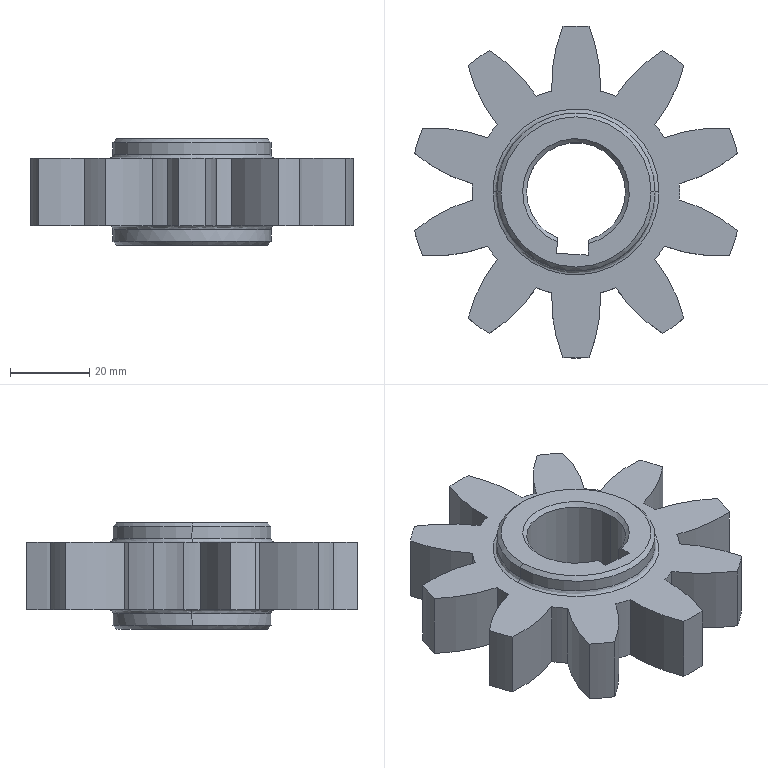Part | SolidWorks | features BaseBody 1 | 1 solid | 69 faces | box 81.679 x 84 x 27 mm | volume 63908 mm3 | cylinder 50 | cone 8 | plane 7 | spline 4 | commonest cylinder face diameters 76.673 x22 52.5 x11 84 x10 40 x4 25 x3